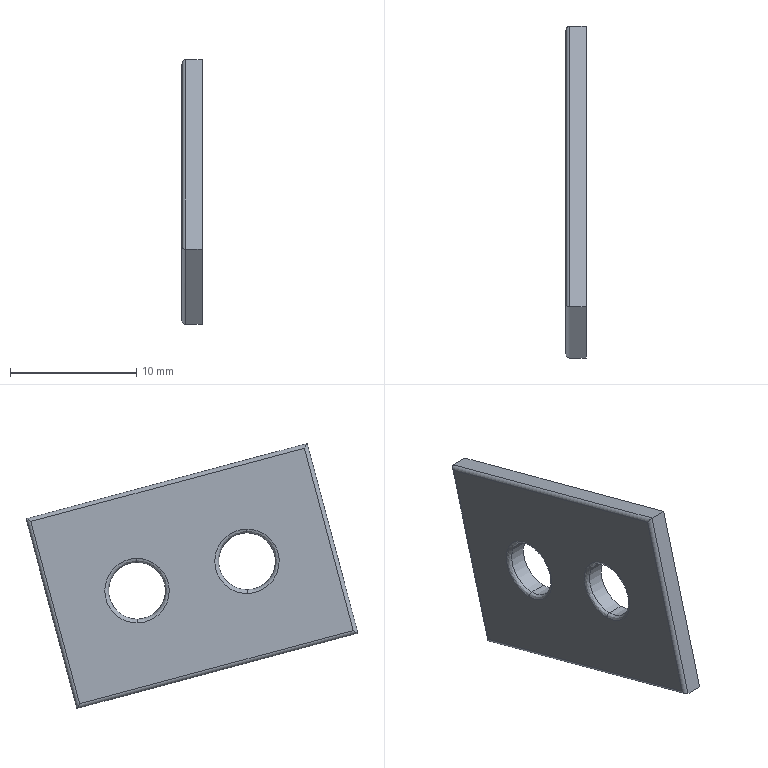Part | STEP file | Guide wheel mechanism revised.sldasm-Part-507 | 1 solid | 18 faces | box 1.6 x 26.233 x 20.944 mm | volume 518.202 mm3 | cylinder 8 | plane 6 | spline 4 | commonest cylinder face diameters 0.6 x4 4.5 x4
STEP:
#1=CARTESIAN_POINT('',(-1.3,8.693,-4.579));
#2=VERTEX_POINT('',#1);
#3=CARTESIAN_POINT('',(-1.3,8.699,-0.07938));
#4=VERTEX_POINT('',#3);
#5=CARTESIAN_POINT('',(-1.3,8.693,-2.329));
#6=DIRECTION('',(1.,0.,0.));
#7=DIRECTION('',(0.,0.,1.));
#8=AXIS2_PLACEMENT_3D('',#5,#6,#7);
#9=CIRCLE('',#8,2.25);
#10=EDGE_CURVE('',#2,#4,#9,.T.);
#11=ORIENTED_EDGE('',*,*,#10,.T.);
#12=CARTESIAN_POINT('',(-1.6,8.7,0.2206));
#13=VERTEX_POINT('',#12);
#14=CARTESIAN_POINT('',(-1.3,8.7,0.2206));
#15=DIRECTION('',(0.,1.,-0.002719));
#16=DIRECTION('',(0.,0.002719,1.));
#17=AXIS2_PLACEMENT_3D('',#14,#15,#16);
#18=CIRCLE('',#17,0.3);
#19=EDGE_CURVE('',#4,#13,#18,.T.);
#20=ORIENTED_EDGE('',*,*,#19,.T.);
#21=CARTESIAN_POINT('',(-1.6,8.693,-4.879));
#22=VERTEX_POINT('',#21);
#23=CARTESIAN_POINT('',(-1.6,8.7,0.2206));
#24=CARTESIAN_POINT('',(-1.6,13.786,0.2068));
#25=CARTESIAN_POINT('',(-1.6,13.779,-4.879));
#26=CARTESIAN_POINT('',(-1.6,8.693,-4.879));
#27=(BOUNDED_CURVE()B_SPLINE_CURVE(3,(#23,#24,#25,#26),.UNSPECIFIED.,.F.,.F.)B_SPLINE_CURVE_WITH_KNOTS((4,4),(0.0008654,1.),.UNSPECIFIED.)CURVE()GEOMETRIC_REPRESENTATION_ITEM()RATIONAL_B_SPLINE_CURVE((1.,0.3342,0.3342,1.))REPRESENTATION_ITEM(''));
#28=EDGE_CURVE('',#13,#22,#27,.T.);
#29=ORIENTED_EDGE('',*,*,#28,.T.);
#30=CARTESIAN_POINT('',(-1.6,8.686,-4.879));
#31=VERTEX_POINT('',#30);
#32=CARTESIAN_POINT('',(-1.6,8.693,-4.879));
#33=CARTESIAN_POINT('',(-1.6,8.691,-4.879));
#34=CARTESIAN_POINT('',(-1.6,8.689,-4.879));
#35=CARTESIAN_POINT('',(-1.6,8.686,-4.879));
#36=B_SPLINE_CURVE_WITH_KNOTS('',3,(#32,#33,#34,#35),.UNSPECIFIED.,.F.,.F.,(4,4),(0.,0.0008545),.UNSPECIFIED.);
#37=EDGE_CURVE('',#22,#31,#36,.T.);
#38=ORIENTED_EDGE('',*,*,#37,.T.);
#39=CARTESIAN_POINT('',(-1.3,8.687,-4.579));
#40=VERTEX_POINT('',#39);
#41=CARTESIAN_POINT('',(-1.3,8.686,-4.879));
#42=DIRECTION('',(0.,-1.,0.002719));
#43=DIRECTION('',(0.,-0.002719,-1.));
#44=AXIS2_PLACEMENT_3D('',#41,#42,#43);
#45=CIRCLE('',#44,0.3);
#46=EDGE_CURVE('',#40,#31,#45,.T.);
#47=ORIENTED_EDGE('',*,*,#46,.F.);
#48=CARTESIAN_POINT('',(-1.3,8.693,-2.329));
#49=DIRECTION('',(1.,0.,0.));
#50=DIRECTION('',(0.,0.,1.));
#51=AXIS2_PLACEMENT_3D('',#48,#49,#50);
#52=CIRCLE('',#51,2.25);
#53=EDGE_CURVE('',#40,#2,#52,.T.);
#54=ORIENTED_EDGE('',*,*,#53,.T.);
#55=EDGE_LOOP('',(#11,#20,#29,#38,#47,#54));
#56=FACE_OUTER_BOUND('',#55,.T.);
#57=CARTESIAN_POINT('',(-1.3,8.699,-0.07938));
#58=CARTESIAN_POINT('',(-1.3,10.017,-0.08296));
#59=CARTESIAN_POINT('',(-1.3,10.947,-1.017));
#60=CARTESIAN_POINT('',(-1.3,10.943,-2.335));
#61=CARTESIAN_POINT('',(-1.3,10.94,-3.654));
#62=CARTESIAN_POINT('',(-1.3,10.005,-4.583));
#63=CARTESIAN_POINT('',(-1.3,8.687,-4.579));
#64=CARTESIAN_POINT('',(-1.477,8.699,-0.07938));
#65=CARTESIAN_POINT('',(-1.477,10.017,-0.08296));
#66=CARTESIAN_POINT('',(-1.477,10.947,-1.017));
#67=CARTESIAN_POINT('',(-1.477,10.943,-2.335));
#68=CARTESIAN_POINT('',(-1.477,10.94,-3.654));
#69=CARTESIAN_POINT('',(-1.477,10.005,-4.583));
#70=CARTESIAN_POINT('',(-1.477,8.687,-4.579));
#71=CARTESIAN_POINT('',(-1.602,8.7,0.0464));
#72=CARTESIAN_POINT('',(-1.602,10.091,0.04262));
#73=CARTESIAN_POINT('',(-1.602,11.073,-0.9441));
#74=CARTESIAN_POINT('',(-1.602,11.069,-2.336));
#75=CARTESIAN_POINT('',(-1.602,11.065,-3.728));
#76=CARTESIAN_POINT('',(-1.602,10.079,-4.709));
#77=CARTESIAN_POINT('',(-1.602,8.687,-4.705));
#78=CARTESIAN_POINT('',(-1.6,8.7,0.2234));
#79=CARTESIAN_POINT('',(-1.6,10.196,0.2194));
#80=CARTESIAN_POINT('',(-1.6,11.25,-0.8409));
#81=CARTESIAN_POINT('',(-1.6,11.246,-2.336));
#82=CARTESIAN_POINT('',(-1.6,11.242,-3.832));
#83=CARTESIAN_POINT('',(-1.6,10.182,-4.886));
#84=CARTESIAN_POINT('',(-1.6,8.686,-4.882));
#85=(BOUNDED_SURFACE()B_SPLINE_SURFACE(3,3,((#57,#58,#59,#60,#61,#62,#63),(#64,#65,#66,#67,#68,#69,#70),(#71,#72,#73,#74,#75,#76,#77),(#78,#79,#80,#81,#82,#83,#84)),.UNSPECIFIED.,.F.,.F.,.F.)B_SPLINE_SURFACE_WITH_KNOTS((4,4),(4,3,4),(0.,1.),(0.,0.5,1.),.UNSPECIFIED.)GEOMETRIC_REPRESENTATION_ITEM()RATIONAL_B_SPLINE_SURFACE(((1.,0.8047,0.8047,1.,0.8047,0.8047,1.),(0.8025,0.6458,0.6458,0.8025,0.6458,0.6458,0.8025),(0.8025,0.6458,0.6458,0.8025,0.6458,0.6458,0.8025),(1.,0.8047,0.8047,1.,0.8047,0.8047,1.)))REPRESENTATION_ITEM('')SURFACE());
#86=ADVANCED_FACE('',(#56),#85,.T.);
#87=CARTESIAN_POINT('',(-1.3,0.,-2.25));
#88=VERTEX_POINT('',#87);
#89=CARTESIAN_POINT('',(-1.3,0.006117,2.25));
#90=VERTEX_POINT('',#89);
#91=CARTESIAN_POINT('',(-1.3,0.,0.));
#92=DIRECTION('',(1.,0.,0.));
#93=DIRECTION('',(0.,0.,1.));
#94=AXIS2_PLACEMENT_3D('',#91,#92,#93);
#95=CIRCLE('',#94,2.25);
#96=EDGE_CURVE('',#88,#90,#95,.T.);
#97=ORIENTED_EDGE('',*,*,#96,.T.);
#98=CARTESIAN_POINT('',(-1.6,0.006933,2.55));
#99=VERTEX_POINT('',#98);
#100=CARTESIAN_POINT('',(-1.3,0.006933,2.55));
#101=DIRECTION('',(0.,1.,-0.002719));
#102=DIRECTION('',(0.,0.002719,1.));
#103=AXIS2_PLACEMENT_3D('',#100,#101,#102);
#104=CIRCLE('',#103,0.3);
#105=EDGE_CURVE('',#90,#99,#104,.T.);
#106=ORIENTED_EDGE('',*,*,#105,.T.);
#107=CARTESIAN_POINT('',(-1.6,0.,-2.55));
#108=VERTEX_POINT('',#107);
#109=CARTESIAN_POINT('',(-1.6,0.006933,2.55));
#110=CARTESIAN_POINT('',(-1.6,5.093,2.536));
#111=CARTESIAN_POINT('',(-1.6,5.086,-2.55));
#112=CARTESIAN_POINT('',(-1.6,0.,-2.55));
#113=(BOUNDED_CURVE()B_SPLINE_CURVE(3,(#109,#110,#111,#112),.UNSPECIFIED.,.F.,.F.)B_SPLINE_CURVE_WITH_KNOTS((4,4),(0.0008654,1.),.UNSPECIFIED.)CURVE()GEOMETRIC_REPRESENTATION_ITEM()RATIONAL_B_SPLINE_CURVE((1.,0.3342,0.3342,1.))REPRESENTATION_ITEM(''));
#114=EDGE_CURVE('',#99,#108,#113,.T.);
#115=ORIENTED_EDGE('',*,*,#114,.T.);
#116=CARTESIAN_POINT('',(-1.6,-0.006933,-2.55));
#117=VERTEX_POINT('',#116);
#118=CARTESIAN_POINT('',(-1.6,0.,-2.55));
#119=CARTESIAN_POINT('',(-1.6,-0.002296,-2.55));
#120=CARTESIAN_POINT('',(-1.6,-0.004651,-2.55));
#121=CARTESIAN_POINT('',(-1.6,-0.006933,-2.55));
#122=B_SPLINE_CURVE_WITH_KNOTS('',3,(#118,#119,#120,#121),.UNSPECIFIED.,.F.,.F.,(4,4),(0.,0.0008545),.UNSPECIFIED.);
#123=EDGE_CURVE('',#108,#117,#122,.T.);
#124=ORIENTED_EDGE('',*,*,#123,.T.);
#125=CARTESIAN_POINT('',(-1.3,-0.006117,-2.25));
#126=VERTEX_POINT('',#125);
#127=CARTESIAN_POINT('',(-1.3,-0.006933,-2.55));
#128=DIRECTION('',(0.,-1.,0.002719));
#129=DIRECTION('',(0.,-0.002719,-1.));
#130=AXIS2_PLACEMENT_3D('',#127,#128,#129);
#131=CIRCLE('',#130,0.3);
#132=EDGE_CURVE('',#126,#117,#131,.T.);
#133=ORIENTED_EDGE('',*,*,#132,.F.);
#134=CARTESIAN_POINT('',(-1.3,0.,0.));
#135=DIRECTION('',(1.,0.,0.));
#136=DIRECTION('',(0.,0.,1.));
#137=AXIS2_PLACEMENT_3D('',#134,#135,#136);
#138=CIRCLE('',#137,2.25);
#139=EDGE_CURVE('',#126,#88,#138,.T.);
#140=ORIENTED_EDGE('',*,*,#139,.T.);
#141=EDGE_LOOP('',(#97,#106,#115,#124,#133,#140));
#142=FACE_OUTER_BOUND('',#141,.T.);
#143=CARTESIAN_POINT('',(-1.3,0.006117,2.25));
#144=CARTESIAN_POINT('',(-1.3,1.324,2.246));
#145=CARTESIAN_POINT('',(-1.3,2.254,1.312));
#146=CARTESIAN_POINT('',(-1.3,2.25,-0.006117));
#147=CARTESIAN_POINT('',(-1.3,2.246,-1.324));
#148=CARTESIAN_POINT('',(-1.3,1.312,-2.254));
#149=CARTESIAN_POINT('',(-1.3,-0.006117,-2.25));
#150=CARTESIAN_POINT('',(-1.477,0.006117,2.25));
#151=CARTESIAN_POINT('',(-1.477,1.324,2.246));
#152=CARTESIAN_POINT('',(-1.477,2.254,1.312));
#153=CARTESIAN_POINT('',(-1.477,2.25,-0.006117));
#154=CARTESIAN_POINT('',(-1.477,2.246,-1.324));
#155=CARTESIAN_POINT('',(-1.477,1.312,-2.254));
#156=CARTESIAN_POINT('',(-1.477,-0.006117,-2.25));
#157=CARTESIAN_POINT('',(-1.602,0.006459,2.376));
#158=CARTESIAN_POINT('',(-1.602,1.398,2.372));
#159=CARTESIAN_POINT('',(-1.602,2.38,1.385));
#160=CARTESIAN_POINT('',(-1.602,2.376,-0.006459));
#161=CARTESIAN_POINT('',(-1.602,2.372,-1.398));
#162=CARTESIAN_POINT('',(-1.602,1.385,-2.38));
#163=CARTESIAN_POINT('',(-1.602,-0.006459,-2.376));
#164=CARTESIAN_POINT('',(-1.6,0.00694,2.553));
#165=CARTESIAN_POINT('',(-1.6,1.502,2.549));
#166=CARTESIAN_POINT('',(-1.6,2.557,1.488));
#167=CARTESIAN_POINT('',(-1.6,2.553,-0.00694));
#168=CARTESIAN_POINT('',(-1.6,2.549,-1.502));
#169=CARTESIAN_POINT('',(-1.6,1.488,-2.557));
#170=CARTESIAN_POINT('',(-1.6,-0.00694,-2.553));
#171=(BOUNDED_SURFACE()B_SPLINE_SURFACE(3,3,((#143,#144,#145,#146,#147,#148,#149),(#150,#151,#152,#153,#154,#155,#156),(#157,#158,#159,#160,#161,#162,#163),(#164,#165,#166,#167,#168,#169,#170)),.UNSPECIFIED.,.F.,.F.,.F.)B_SPLINE_SURFACE_WITH_KNOTS((4,4),(4,3,4),(0.,1.),(0.,0.5,1.),.UNSPECIFIED.)GEOMETRIC_REPRESENTATION_ITEM()RATIONAL_B_SPLINE_SURFACE(((1.,0.8047,0.8047,1.,0.8047,0.8047,1.),(0.8025,0.6458,0.6458,0.8025,0.6458,0.6458,0.8025),(0.8025,0.6458,0.6458,0.8025,0.6458,0.6458,0.8025),(1.,0.8047,0.8047,1.,0.8047,0.8047,1.)))REPRESENTATION_ITEM('')SURFACE());
#172=ADVANCED_FACE('',(#142),#171,.T.);
#173=CARTESIAN_POINT('',(0.,8.693,-0.07937));
#174=VERTEX_POINT('',#173);
#175=CARTESIAN_POINT('',(0.,8.693,-4.579));
#176=VERTEX_POINT('',#175);
#177=CARTESIAN_POINT('',(0.,8.693,-2.329));
#178=DIRECTION('',(1.,0.,0.));
#179=DIRECTION('',(0.,0.,1.));
#180=AXIS2_PLACEMENT_3D('',#177,#178,#179);
#181=CIRCLE('',#180,2.25);
#182=EDGE_CURVE('',#174,#176,#181,.T.);
#183=ORIENTED_EDGE('',*,*,#182,.T.);
#184=CARTESIAN_POINT('',(0.,8.693,-4.579));
#185=DIRECTION('',(-1.,0.,0.));
#186=VECTOR('',#185,1000.);
#187=LINE('',#184,#186);
#188=EDGE_CURVE('',#176,#2,#187,.T.);
#189=ORIENTED_EDGE('',*,*,#188,.T.);
#190=ORIENTED_EDGE('',*,*,#53,.F.);
#191=CARTESIAN_POINT('',(-1.3,8.693,-0.07937));
#192=VERTEX_POINT('',#191);
#193=CARTESIAN_POINT('',(-1.3,8.693,-2.329));
#194=DIRECTION('',(1.,0.,0.));
#195=DIRECTION('',(0.,0.,1.));
#196=AXIS2_PLACEMENT_3D('',#193,#194,#195);
#197=CIRCLE('',#196,2.25);
#198=EDGE_CURVE('',#192,#40,#197,.T.);
#199=ORIENTED_EDGE('',*,*,#198,.F.);
#200=CARTESIAN_POINT('',(0.,8.693,-0.07937));
#201=DIRECTION('',(-1.,0.,0.));
#202=VECTOR('',#201,1000.);
#203=LINE('',#200,#202);
#204=EDGE_CURVE('',#174,#192,#203,.T.);
#205=ORIENTED_EDGE('',*,*,#204,.F.);
#206=EDGE_LOOP('',(#183,#189,#190,#199,#205));
#207=FACE_OUTER_BOUND('',#206,.T.);
#208=CARTESIAN_POINT('',(0.,8.693,-2.329));
#209=DIRECTION('',(-1.,0.,0.));
#210=DIRECTION('',(0.,0.,1.));
#211=AXIS2_PLACEMENT_3D('',#208,#209,#210);
#212=CYLINDRICAL_SURFACE('',#211,2.25);
#213=ADVANCED_FACE('',(#207),#212,.F.);
#214=CARTESIAN_POINT('',(0.,0.,2.25));
#215=VERTEX_POINT('',#214);
#216=CARTESIAN_POINT('',(0.,0.,-2.25));
#217=VERTEX_POINT('',#216);
#218=CARTESIAN_POINT('',(0.,0.,0.));
#219=DIRECTION('',(1.,0.,0.));
#220=DIRECTION('',(0.,0.,1.));
#221=AXIS2_PLACEMENT_3D('',#218,#219,#220);
#222=CIRCLE('',#221,2.25);
#223=EDGE_CURVE('',#215,#217,#222,.T.);
#224=ORIENTED_EDGE('',*,*,#223,.T.);
#225=CARTESIAN_POINT('',(0.,0.,-2.25));
#226=DIRECTION('',(-1.,0.,0.));
#227=VECTOR('',#226,1000.);
#228=LINE('',#225,#227);
#229=EDGE_CURVE('',#217,#88,#228,.T.);
#230=ORIENTED_EDGE('',*,*,#229,.T.);
#231=ORIENTED_EDGE('',*,*,#139,.F.);
#232=CARTESIAN_POINT('',(-1.3,0.,2.25));
#233=VERTEX_POINT('',#232);
#234=CARTESIAN_POINT('',(-1.3,0.,0.));
#235=DIRECTION('',(1.,0.,0.));
#236=DIRECTION('',(0.,0.,1.));
#237=AXIS2_PLACEMENT_3D('',#234,#235,#236);
#238=CIRCLE('',#237,2.25);
#239=EDGE_CURVE('',#233,#126,#238,.T.);
#240=ORIENTED_EDGE('',*,*,#239,.F.);
#241=CARTESIAN_POINT('',(0.,0.,2.25));
#242=DIRECTION('',(-1.,0.,0.));
#243=VECTOR('',#242,1000.);
#244=LINE('',#241,#243);
#245=EDGE_CURVE('',#215,#233,#244,.T.);
#246=ORIENTED_EDGE('',*,*,#245,.F.);
#247=EDGE_LOOP('',(#224,#230,#231,#240,#246));
#248=FACE_OUTER_BOUND('',#247,.T.);
#249=CARTESIAN_POINT('',(0.,0.,0.));
#250=DIRECTION('',(-1.,0.,0.));
#251=DIRECTION('',(0.,0.,1.));
#252=AXIS2_PLACEMENT_3D('',#249,#250,#251);
#253=CYLINDRICAL_SURFACE('',#252,2.25);
#254=ADVANCED_FACE('',(#248),#253,.F.);
#255=ORIENTED_EDGE('',*,*,#182,.F.);
#256=CARTESIAN_POINT('',(0.,8.693,-2.329));
#257=DIRECTION('',(1.,0.,0.));
#258=DIRECTION('',(0.,0.,1.));
#259=AXIS2_PLACEMENT_3D('',#256,#257,#258);
#260=CIRCLE('',#259,2.25);
#261=EDGE_CURVE('',#176,#174,#260,.T.);
#262=ORIENTED_EDGE('',*,*,#261,.F.);
#263=EDGE_LOOP('',(#255,#262));
#264=FACE_BOUND('',#263,.T.);
#265=ORIENTED_EDGE('',*,*,#223,.F.);
#266=CARTESIAN_POINT('',(0.,0.,0.));
#267=DIRECTION('',(1.,0.,0.));
#268=DIRECTION('',(0.,0.,1.));
#269=AXIS2_PLACEMENT_3D('',#266,#267,#268);
#270=CIRCLE('',#269,2.25);
#271=EDGE_CURVE('',#217,#215,#270,.T.);
#272=ORIENTED_EDGE('',*,*,#271,.F.);
#273=EDGE_LOOP('',(#265,#272));
#274=FACE_BOUND('',#273,.T.);
#275=CARTESIAN_POINT('',(0.,-4.753,9.307));
#276=VERTEX_POINT('',#275);
#277=CARTESIAN_POINT('',(0.,17.463,3.354));
#278=VERTEX_POINT('',#277);
#279=CARTESIAN_POINT('',(0.,-4.753,9.307));
#280=DIRECTION('',(0.,0.9659,-0.2588));
#281=VECTOR('',#280,1000.);
#282=LINE('',#279,#281);
#283=EDGE_CURVE('',#276,#278,#282,.T.);
#284=ORIENTED_EDGE('',*,*,#283,.F.);
#285=CARTESIAN_POINT('',(0.,-8.77,-5.684));
#286=VERTEX_POINT('',#285);
#287=CARTESIAN_POINT('',(0.,-8.77,-5.684));
#288=DIRECTION('',(0.,0.2588,0.9659));
#289=VECTOR('',#288,1000.);
#290=LINE('',#287,#289);
#291=EDGE_CURVE('',#286,#276,#290,.T.);
#292=ORIENTED_EDGE('',*,*,#291,.F.);
#293=CARTESIAN_POINT('',(0.,13.446,-11.637));
#294=VERTEX_POINT('',#293);
#295=CARTESIAN_POINT('',(0.,13.446,-11.637));
#296=DIRECTION('',(0.,-0.9659,0.2588));
#297=VECTOR('',#296,1000.);
#298=LINE('',#295,#297);
#299=EDGE_CURVE('',#294,#286,#298,.T.);
#300=ORIENTED_EDGE('',*,*,#299,.F.);
#301=CARTESIAN_POINT('',(0.,17.463,3.354));
#302=DIRECTION('',(0.,-0.2588,-0.9659));
#303=VECTOR('',#302,1000.);
#304=LINE('',#301,#303);
#305=EDGE_CURVE('',#278,#294,#304,.T.);
#306=ORIENTED_EDGE('',*,*,#305,.F.);
#307=EDGE_LOOP('',(#284,#292,#300,#306));
#308=FACE_OUTER_BOUND('',#307,.T.);
#309=CARTESIAN_POINT('',(0.,0.,0.));
#310=DIRECTION('',(-1.,0.,0.));
#311=DIRECTION('',(0.,0.,1.));
#312=AXIS2_PLACEMENT_3D('',#309,#310,#311);
#313=PLANE('',#312);
#314=ADVANCED_FACE('',(#264,#274,#308),#313,.F.);
#315=ORIENTED_EDGE('',*,*,#188,.F.);
#316=ORIENTED_EDGE('',*,*,#261,.T.);
#317=ORIENTED_EDGE('',*,*,#204,.T.);
#318=CARTESIAN_POINT('',(-1.3,8.693,-2.329));
#319=DIRECTION('',(1.,0.,0.));
#320=DIRECTION('',(0.,0.,1.));
#321=AXIS2_PLACEMENT_3D('',#318,#319,#320);
#322=CIRCLE('',#321,2.25);
#323=EDGE_CURVE('',#4,#192,#322,.T.);
#324=ORIENTED_EDGE('',*,*,#323,.F.);
#325=ORIENTED_EDGE('',*,*,#10,.F.);
#326=EDGE_LOOP('',(#315,#316,#317,#324,#325));
#327=FACE_OUTER_BOUND('',#326,.T.);
#328=CARTESIAN_POINT('',(0.,8.693,-2.329));
#329=DIRECTION('',(-1.,0.,0.));
#330=DIRECTION('',(0.,0.,1.));
#331=AXIS2_PLACEMENT_3D('',#328,#329,#330);
#332=CYLINDRICAL_SURFACE('',#331,2.25);
#333=ADVANCED_FACE('',(#327),#332,.F.);
#334=ORIENTED_EDGE('',*,*,#229,.F.);
#335=ORIENTED_EDGE('',*,*,#271,.T.);
#336=ORIENTED_EDGE('',*,*,#245,.T.);
#337=CARTESIAN_POINT('',(-1.3,0.,0.));
#338=DIRECTION('',(1.,0.,0.));
#339=DIRECTION('',(0.,0.,1.));
#340=AXIS2_PLACEMENT_3D('',#337,#338,#339);
#341=CIRCLE('',#340,2.25);
#342=EDGE_CURVE('',#90,#233,#341,.T.);
#343=ORIENTED_EDGE('',*,*,#342,.F.);
#344=ORIENTED_EDGE('',*,*,#96,.F.);
#345=EDGE_LOOP('',(#334,#335,#336,#343,#344));
#346=FACE_OUTER_BOUND('',#345,.T.);
#347=CARTESIAN_POINT('',(0.,0.,0.));
#348=DIRECTION('',(-1.,0.,0.));
#349=DIRECTION('',(0.,0.,1.));
#350=AXIS2_PLACEMENT_3D('',#347,#348,#349);
#351=CYLINDRICAL_SURFACE('',#350,2.25);
#352=ADVANCED_FACE('',(#346),#351,.F.);
#353=CARTESIAN_POINT('',(-1.3,13.446,-11.637));
#354=VERTEX_POINT('',#353);
#355=CARTESIAN_POINT('',(0.,13.446,-11.637));
#356=DIRECTION('',(-1.,0.,0.));
#357=VECTOR('',#356,1000.);
#358=LINE('',#355,#357);
#359=EDGE_CURVE('',#294,#354,#358,.T.);
#360=ORIENTED_EDGE('',*,*,#359,.T.);
#361=CARTESIAN_POINT('',(-1.3,17.463,3.354));
#362=VERTEX_POINT('',#361);
#363=CARTESIAN_POINT('',(-1.3,17.463,3.354));
#364=DIRECTION('',(0.,0.2588,0.9659));
#365=VECTOR('',#364,1000.);
#366=LINE('',#363,#365);
#367=EDGE_CURVE('',#354,#362,#366,.T.);
#368=ORIENTED_EDGE('',*,*,#367,.T.);
#369=CARTESIAN_POINT('',(0.,17.463,3.354));
#370=DIRECTION('',(1.,0.,0.));
#371=VECTOR('',#370,1000.);
#372=LINE('',#369,#371);
#373=EDGE_CURVE('',#362,#278,#372,.T.);
#374=ORIENTED_EDGE('',*,*,#373,.T.);
#375=ORIENTED_EDGE('',*,*,#305,.T.);
#376=EDGE_LOOP('',(#360,#368,#374,#375));
#377=FACE_OUTER_BOUND('',#376,.T.);
#378=CARTESIAN_POINT('',(0.,17.463,3.354));
#379=DIRECTION('',(0.,0.9659,-0.2588));
#380=DIRECTION('',(0.,0.2588,0.9659));
#381=AXIS2_PLACEMENT_3D('',#378,#379,#380);
#382=PLANE('',#381);
#383=ADVANCED_FACE('',(#377),#382,.T.);
#384=ORIENTED_EDGE('',*,*,#373,.F.);
#385=CARTESIAN_POINT('',(-1.3,-4.753,9.307));
#386=VERTEX_POINT('',#385);
#387=CARTESIAN_POINT('',(-1.3,-4.753,9.307));
#388=DIRECTION('',(0.,-0.9659,0.2588));
#389=VECTOR('',#388,1000.);
#390=LINE('',#387,#389);
#391=EDGE_CURVE('',#362,#386,#390,.T.);
#392=ORIENTED_EDGE('',*,*,#391,.T.);
#393=CARTESIAN_POINT('',(0.,-4.753,9.307));
#394=DIRECTION('',(1.,0.,0.));
#395=VECTOR('',#394,1000.);
#396=LINE('',#393,#395);
#397=EDGE_CURVE('',#386,#276,#396,.T.);
#398=ORIENTED_EDGE('',*,*,#397,.T.);
#399=ORIENTED_EDGE('',*,*,#283,.T.);
#400=EDGE_LOOP('',(#384,#392,#398,#399));
#401=FACE_OUTER_BOUND('',#400,.T.);
#402=CARTESIAN_POINT('',(0.,-4.753,9.307));
#403=DIRECTION('',(0.,0.2588,0.9659));
#404=DIRECTION('',(0.,-0.9659,0.2588));
#405=AXIS2_PLACEMENT_3D('',#402,#403,#404);
#406=PLANE('',#405);
#407=ADVANCED_FACE('',(#401),#406,.T.);
#408=ORIENTED_EDGE('',*,*,#397,.F.);
#409=CARTESIAN_POINT('',(-1.3,-8.77,-5.684));
#410=VERTEX_POINT('',#409);
#411=CARTESIAN_POINT('',(-1.3,-8.77,-5.684));
#412=DIRECTION('',(0.,-0.2588,-0.9659));
#413=VECTOR('',#412,1000.);
#414=LINE('',#411,#413);
#415=EDGE_CURVE('',#386,#410,#414,.T.);
#416=ORIENTED_EDGE('',*,*,#415,.T.);
#417=CARTESIAN_POINT('',(0.,-8.77,-5.684));
#418=DIRECTION('',(1.,0.,0.));
#419=VECTOR('',#418,1000.);
#420=LINE('',#417,#419);
#421=EDGE_CURVE('',#410,#286,#420,.T.);
#422=ORIENTED_EDGE('',*,*,#421,.T.);
#423=ORIENTED_EDGE('',*,*,#291,.T.);
#424=EDGE_LOOP('',(#408,#416,#422,#423));
#425=FACE_OUTER_BOUND('',#424,.T.);
#426=CARTESIAN_POINT('',(0.,-8.77,-5.684));
#427=DIRECTION('',(0.,-0.9659,0.2588));
#428=DIRECTION('',(0.,-0.2588,-0.9659));
#429=AXIS2_PLACEMENT_3D('',#426,#427,#428);
#430=PLANE('',#429);
#431=ADVANCED_FACE('',(#425),#430,.T.);
#432=ORIENTED_EDGE('',*,*,#421,.F.);
#433=CARTESIAN_POINT('',(-1.3,13.446,-11.637));
#434=DIRECTION('',(0.,0.9659,-0.2588));
#435=VECTOR('',#434,1000.);
#436=LINE('',#433,#435);
#437=EDGE_CURVE('',#410,#354,#436,.T.);
#438=ORIENTED_EDGE('',*,*,#437,.T.);
#439=ORIENTED_EDGE('',*,*,#359,.F.);
#440=ORIENTED_EDGE('',*,*,#299,.T.);
#441=EDGE_LOOP('',(#432,#438,#439,#440));
#442=FACE_OUTER_BOUND('',#441,.T.);
#443=CARTESIAN_POINT('',(0.,13.446,-11.637));
#444=DIRECTION('',(0.,-0.2588,-0.9659));
#445=DIRECTION('',(0.,0.9659,-0.2588));
#446=AXIS2_PLACEMENT_3D('',#443,#444,#445);
#447=PLANE('',#446);
#448=ADVANCED_FACE('',(#442),#447,.T.);
#449=ORIENTED_EDGE('',*,*,#19,.F.);
#450=ORIENTED_EDGE('',*,*,#323,.T.);
#451=ORIENTED_EDGE('',*,*,#198,.T.);
#452=ORIENTED_EDGE('',*,*,#46,.T.);
#453=CARTESIAN_POINT('',(-1.6,8.693,0.2206));
#454=VERTEX_POINT('',#453);
#455=CARTESIAN_POINT('',(-1.6,8.686,-4.879));
#456=CARTESIAN_POINT('',(-1.6,8.353,-4.878));
#457=CARTESIAN_POINT('',(-1.6,8.02,-4.811));
#458=CARTESIAN_POINT('',(-1.6,7.404,-4.555));
#459=CARTESIAN_POINT('',(-1.6,7.122,-4.365));
#460=CARTESIAN_POINT('',(-1.6,6.651,-3.893));
#461=CARTESIAN_POINT('',(-1.6,6.463,-3.61));
#462=CARTESIAN_POINT('',(-1.6,6.209,-2.993));
#463=CARTESIAN_POINT('',(-1.6,6.143,-2.659));
#464=CARTESIAN_POINT('',(-1.6,6.144,-1.992));
#465=CARTESIAN_POINT('',(-1.6,6.21,-1.659));
#466=CARTESIAN_POINT('',(-1.6,6.466,-1.043));
#467=CARTESIAN_POINT('',(-1.6,6.655,-0.7606));
#468=CARTESIAN_POINT('',(-1.6,7.127,-0.2893));
#469=CARTESIAN_POINT('',(-1.6,7.41,-0.1006));
#470=CARTESIAN_POINT('',(-1.6,8.026,0.1544));
#471=CARTESIAN_POINT('',(-1.6,8.36,0.2206));
#472=CARTESIAN_POINT('',(-1.6,8.693,0.2206));
#473=B_SPLINE_CURVE_WITH_KNOTS('',3,(#455,#456,#457,#458,#459,#460,#461,#462,#463,#464,#465,#466,#467,#468,#469,#470,#471,#472),.UNSPECIFIED.,.F.,.F.,(4,2,2,2,2,2,2,2,4),(0.0008545,0.1257,0.2506,0.3755,0.5004,0.6253,0.7502,0.8751,1.),.UNSPECIFIED.);
#474=EDGE_CURVE('',#31,#454,#473,.T.);
#475=ORIENTED_EDGE('',*,*,#474,.T.);
#476=CARTESIAN_POINT('',(-1.6,8.693,0.2206));
#477=CARTESIAN_POINT('',(-1.6,8.696,0.2206));
#478=CARTESIAN_POINT('',(-1.6,8.698,0.2206));
#479=CARTESIAN_POINT('',(-1.6,8.7,0.2206));
#480=(BOUNDED_CURVE()B_SPLINE_CURVE(3,(#476,#477,#478,#479),.UNSPECIFIED.,.F.,.F.)B_SPLINE_CURVE_WITH_KNOTS((4,4),(0.,0.0008654),.UNSPECIFIED.)CURVE()GEOMETRIC_REPRESENTATION_ITEM()RATIONAL_B_SPLINE_CURVE((1.,1.,1.,1.))REPRESENTATION_ITEM(''));
#481=EDGE_CURVE('',#454,#13,#480,.T.);
#482=ORIENTED_EDGE('',*,*,#481,.T.);
#483=EDGE_LOOP('',(#449,#450,#451,#452,#475,#482));
#484=FACE_OUTER_BOUND('',#483,.T.);
#485=CARTESIAN_POINT('',(-1.3,8.687,-4.579));
#486=CARTESIAN_POINT('',(-1.3,4.187,-4.567));
#487=CARTESIAN_POINT('',(-1.3,4.199,-0.06715));
#488=CARTESIAN_POINT('',(-1.3,8.699,-0.07938));
#489=CARTESIAN_POINT('',(-1.477,8.687,-4.579));
#490=CARTESIAN_POINT('',(-1.477,4.187,-4.567));
#491=CARTESIAN_POINT('',(-1.477,4.199,-0.06715));
#492=CARTESIAN_POINT('',(-1.477,8.699,-0.07938));
#493=CARTESIAN_POINT('',(-1.602,8.687,-4.705));
#494=CARTESIAN_POINT('',(-1.602,3.935,-4.692));
#495=CARTESIAN_POINT('',(-1.602,3.948,0.05945));
#496=CARTESIAN_POINT('',(-1.602,8.7,0.04653));
#497=CARTESIAN_POINT('',(-1.6,8.686,-4.882));
#498=CARTESIAN_POINT('',(-1.6,3.58,-4.869));
#499=CARTESIAN_POINT('',(-1.6,3.594,0.2376));
#500=CARTESIAN_POINT('',(-1.6,8.7,0.2237));
#501=(BOUNDED_SURFACE()B_SPLINE_SURFACE(3,3,((#485,#486,#487,#488),(#489,#490,#491,#492),(#493,#494,#495,#496),(#497,#498,#499,#500)),.UNSPECIFIED.,.F.,.F.,.T.)B_SPLINE_SURFACE_WITH_KNOTS((4,4),(4,4),(0.,1.),(0.,1.),.UNSPECIFIED.)GEOMETRIC_REPRESENTATION_ITEM()RATIONAL_B_SPLINE_SURFACE(((1.,0.3333,0.3333,1.),(0.8023,0.2674,0.2674,0.8023),(0.8023,0.2674,0.2674,0.8023),(1.,0.3333,0.3333,1.)))REPRESENTATION_ITEM('')SURFACE());
#502=ADVANCED_FACE('',(#484),#501,.T.);
#503=ORIENTED_EDGE('',*,*,#105,.F.);
#504=ORIENTED_EDGE('',*,*,#342,.T.);
#505=ORIENTED_EDGE('',*,*,#239,.T.);
#506=ORIENTED_EDGE('',*,*,#132,.T.);
#507=CARTESIAN_POINT('',(-1.6,0.,2.55));
#508=VERTEX_POINT('',#507);
#509=CARTESIAN_POINT('',(-1.6,-0.006933,-2.55));
#510=CARTESIAN_POINT('',(-1.6,-0.3404,-2.549));
#511=CARTESIAN_POINT('',(-1.6,-0.6736,-2.482));
#512=CARTESIAN_POINT('',(-1.6,-1.289,-2.225));
#513=CARTESIAN_POINT('',(-1.6,-1.571,-2.036));
#514=CARTESIAN_POINT('',(-1.6,-2.042,-1.563));
#515=CARTESIAN_POINT('',(-1.6,-2.231,-1.28));
#516=CARTESIAN_POINT('',(-1.6,-2.485,-0.6635));
#517=CARTESIAN_POINT('',(-1.6,-2.551,-0.3301));
#518=CARTESIAN_POINT('',(-1.6,-2.55,0.337));
#519=CARTESIAN_POINT('',(-1.6,-2.483,0.6703));
#520=CARTESIAN_POINT('',(-1.6,-2.227,1.286));
#521=CARTESIAN_POINT('',(-1.6,-2.038,1.569));
#522=CARTESIAN_POINT('',(-1.6,-1.566,2.04));
#523=CARTESIAN_POINT('',(-1.6,-1.283,2.229));
#524=CARTESIAN_POINT('',(-1.6,-0.6669,2.484));
#525=CARTESIAN_POINT('',(-1.6,-0.3335,2.55));
#526=CARTESIAN_POINT('',(-1.6,0.,2.55));
#527=B_SPLINE_CURVE_WITH_KNOTS('',3,(#509,#510,#511,#512,#513,#514,#515,#516,#517,#518,#519,#520,#521,#522,#523,#524,#525,#526),.UNSPECIFIED.,.F.,.F.,(4,2,2,2,2,2,2,2,4),(0.0008545,0.1257,0.2506,0.3755,0.5004,0.6253,0.7502,0.8751,1.),.UNSPECIFIED.);
#528=EDGE_CURVE('',#117,#508,#527,.T.);
#529=ORIENTED_EDGE('',*,*,#528,.T.);
#530=CARTESIAN_POINT('',(-1.6,0.,2.55));
#531=CARTESIAN_POINT('',(-1.6,0.002311,2.55));
#532=CARTESIAN_POINT('',(-1.6,0.004622,2.55));
#533=CARTESIAN_POINT('',(-1.6,0.006933,2.55));
#534=(BOUNDED_CURVE()B_SPLINE_CURVE(3,(#530,#531,#532,#533),.UNSPECIFIED.,.F.,.F.)B_SPLINE_CURVE_WITH_KNOTS((4,4),(0.,0.0008654),.UNSPECIFIED.)CURVE()GEOMETRIC_REPRESENTATION_ITEM()RATIONAL_B_SPLINE_CURVE((1.,1.,1.,1.))REPRESENTATION_ITEM(''));
#535=EDGE_CURVE('',#508,#99,#534,.T.);
#536=ORIENTED_EDGE('',*,*,#535,.T.);
#537=EDGE_LOOP('',(#503,#504,#505,#506,#529,#536));
#538=FACE_OUTER_BOUND('',#537,.T.);
#539=CARTESIAN_POINT('',(-1.3,-0.006117,-2.25));
#540=CARTESIAN_POINT('',(-1.3,-4.506,-2.238));
#541=CARTESIAN_POINT('',(-1.3,-4.494,2.262));
#542=CARTESIAN_POINT('',(-1.3,0.006117,2.25));
#543=CARTESIAN_POINT('',(-1.477,-0.006117,-2.25));
#544=CARTESIAN_POINT('',(-1.477,-4.506,-2.238));
#545=CARTESIAN_POINT('',(-1.477,-4.494,2.262));
#546=CARTESIAN_POINT('',(-1.477,0.006117,2.25));
#547=CARTESIAN_POINT('',(-1.602,-0.006459,-2.376));
#548=CARTESIAN_POINT('',(-1.602,-4.758,-2.363));
#549=CARTESIAN_POINT('',(-1.602,-4.745,2.389));
#550=CARTESIAN_POINT('',(-1.602,0.006459,2.376));
#551=CARTESIAN_POINT('',(-1.6,-0.006941,-2.553));
#552=CARTESIAN_POINT('',(-1.6,-5.113,-2.539));
#553=CARTESIAN_POINT('',(-1.6,-5.099,2.567));
#554=CARTESIAN_POINT('',(-1.6,0.006941,2.553));
#555=(BOUNDED_SURFACE()B_SPLINE_SURFACE(3,3,((#539,#540,#541,#542),(#543,#544,#545,#546),(#547,#548,#549,#550),(#551,#552,#553,#554)),.UNSPECIFIED.,.F.,.F.,.F.)B_SPLINE_SURFACE_WITH_KNOTS((4,4),(4,4),(0.,1.),(0.,1.),.UNSPECIFIED.)GEOMETRIC_REPRESENTATION_ITEM()RATIONAL_B_SPLINE_SURFACE(((1.,0.3333,0.3333,1.),(0.8023,0.2674,0.2674,0.8023),(0.8023,0.2674,0.2674,0.8023),(1.,0.3333,0.3333,1.)))REPRESENTATION_ITEM('')SURFACE());
#556=ADVANCED_FACE('',(#538),#555,.T.);
#557=CARTESIAN_POINT('',(-1.6,13.234,-11.269));
#558=VERTEX_POINT('',#557);
#559=CARTESIAN_POINT('',(-1.3,13.446,-11.637));
#560=CARTESIAN_POINT('',(-1.476,13.446,-11.637));
#561=CARTESIAN_POINT('',(-1.6,13.359,-11.484));
#562=CARTESIAN_POINT('',(-1.6,13.234,-11.269));
#563=(BOUNDED_CURVE()B_SPLINE_CURVE(3,(#559,#560,#561,#562),.UNSPECIFIED.,.F.,.F.)B_SPLINE_CURVE_WITH_KNOTS((4,4),(0.,1.571),.UNSPECIFIED.)CURVE()GEOMETRIC_REPRESENTATION_ITEM()RATIONAL_B_SPLINE_CURVE((1.,0.8047,0.8047,1.))REPRESENTATION_ITEM(''));
#564=EDGE_CURVE('',#354,#558,#563,.T.);
#565=ORIENTED_EDGE('',*,*,#564,.T.);
#566=CARTESIAN_POINT('',(-1.6,17.096,3.142));
#567=VERTEX_POINT('',#566);
#568=CARTESIAN_POINT('',(-1.6,17.175,3.436));
#569=DIRECTION('',(0.,0.2588,0.9659));
#570=VECTOR('',#569,1000.);
#571=LINE('',#568,#570);
#572=EDGE_CURVE('',#558,#567,#571,.T.);
#573=ORIENTED_EDGE('',*,*,#572,.T.);
#574=CARTESIAN_POINT('',(-1.6,17.096,3.142));
#575=CARTESIAN_POINT('',(-1.6,17.311,3.267));
#576=CARTESIAN_POINT('',(-1.476,17.463,3.354));
#577=CARTESIAN_POINT('',(-1.3,17.463,3.354));
#578=(BOUNDED_CURVE()B_SPLINE_CURVE(3,(#574,#575,#576,#577),.UNSPECIFIED.,.F.,.T.)B_SPLINE_CURVE_WITH_KNOTS((4,4),(1.571,3.142),.UNSPECIFIED.)CURVE()GEOMETRIC_REPRESENTATION_ITEM()RATIONAL_B_SPLINE_CURVE((1.,0.8047,0.8047,1.))REPRESENTATION_ITEM(''));
#579=EDGE_CURVE('',#567,#362,#578,.T.);
#580=ORIENTED_EDGE('',*,*,#579,.T.);
#581=ORIENTED_EDGE('',*,*,#367,.F.);
#582=EDGE_LOOP('',(#565,#573,#580,#581));
#583=FACE_OUTER_BOUND('',#582,.T.);
#584=CARTESIAN_POINT('',(-1.3,17.175,3.436));
#585=DIRECTION('',(0.,-0.2588,-0.9659));
#586=DIRECTION('',(0.,0.9659,-0.2588));
#587=AXIS2_PLACEMENT_3D('',#584,#585,#586);
#588=CYLINDRICAL_SURFACE('',#587,0.3);
#589=ADVANCED_FACE('',(#583),#588,.T.);
#590=CARTESIAN_POINT('',(-1.6,-4.541,8.94));
#591=VERTEX_POINT('',#590);
#592=CARTESIAN_POINT('',(-1.6,-4.541,8.94));
#593=CARTESIAN_POINT('',(-1.6,-4.665,9.155));
#594=CARTESIAN_POINT('',(-1.476,-4.753,9.307));
#595=CARTESIAN_POINT('',(-1.3,-4.753,9.307));
#596=(BOUNDED_CURVE()B_SPLINE_CURVE(3,(#592,#593,#594,#595),.UNSPECIFIED.,.F.,.F.)B_SPLINE_CURVE_WITH_KNOTS((4,4),(1.571,3.142),.UNSPECIFIED.)CURVE()GEOMETRIC_REPRESENTATION_ITEM()RATIONAL_B_SPLINE_CURVE((1.,0.8047,0.8047,1.))REPRESENTATION_ITEM(''));
#597=EDGE_CURVE('',#591,#386,#596,.T.);
#598=ORIENTED_EDGE('',*,*,#597,.T.);
#599=ORIENTED_EDGE('',*,*,#391,.F.);
#600=ORIENTED_EDGE('',*,*,#579,.F.);
#601=CARTESIAN_POINT('',(-1.6,-4.835,9.019));
#602=DIRECTION('',(0.,-0.9659,0.2588));
#603=VECTOR('',#602,1000.);
#604=LINE('',#601,#603);
#605=EDGE_CURVE('',#567,#591,#604,.T.);
#606=ORIENTED_EDGE('',*,*,#605,.T.);
#607=EDGE_LOOP('',(#598,#599,#600,#606));
#608=FACE_OUTER_BOUND('',#607,.T.);
#609=CARTESIAN_POINT('',(-1.3,-4.835,9.019));
#610=DIRECTION('',(0.,0.9659,-0.2588));
#611=DIRECTION('',(0.,0.2588,0.9659));
#612=AXIS2_PLACEMENT_3D('',#609,#610,#611);
#613=CYLINDRICAL_SURFACE('',#612,0.3);
#614=ADVANCED_FACE('',(#608),#613,.T.);
#615=CARTESIAN_POINT('',(-1.6,-8.402,-5.472));
#616=VERTEX_POINT('',#615);
#617=CARTESIAN_POINT('',(-1.6,-8.402,-5.472));
#618=CARTESIAN_POINT('',(-1.6,-8.618,-5.596));
#619=CARTESIAN_POINT('',(-1.476,-8.77,-5.684));
#620=CARTESIAN_POINT('',(-1.3,-8.77,-5.684));
#621=(BOUNDED_CURVE()B_SPLINE_CURVE(3,(#617,#618,#619,#620),.UNSPECIFIED.,.F.,.F.)B_SPLINE_CURVE_WITH_KNOTS((4,4),(1.571,3.142),.UNSPECIFIED.)CURVE()GEOMETRIC_REPRESENTATION_ITEM()RATIONAL_B_SPLINE_CURVE((1.,0.8047,0.8047,1.))REPRESENTATION_ITEM(''));
#622=EDGE_CURVE('',#616,#410,#621,.T.);
#623=ORIENTED_EDGE('',*,*,#622,.T.);
#624=ORIENTED_EDGE('',*,*,#415,.F.);
#625=ORIENTED_EDGE('',*,*,#597,.F.);
#626=CARTESIAN_POINT('',(-1.6,-8.481,-5.766));
#627=DIRECTION('',(0.,-0.2588,-0.9659));
#628=VECTOR('',#627,1000.);
#629=LINE('',#626,#628);
#630=EDGE_CURVE('',#591,#616,#629,.T.);
#631=ORIENTED_EDGE('',*,*,#630,.T.);
#632=EDGE_LOOP('',(#623,#624,#625,#631));
#633=FACE_OUTER_BOUND('',#632,.T.);
#634=CARTESIAN_POINT('',(-1.3,-8.481,-5.766));
#635=DIRECTION('',(0.,0.2588,0.9659));
#636=DIRECTION('',(0.,-0.9659,0.2588));
#637=AXIS2_PLACEMENT_3D('',#634,#635,#636);
#638=CYLINDRICAL_SURFACE('',#637,0.3);
#639=ADVANCED_FACE('',(#633),#638,.T.);
#640=ORIENTED_EDGE('',*,*,#564,.F.);
#641=ORIENTED_EDGE('',*,*,#437,.F.);
#642=ORIENTED_EDGE('',*,*,#622,.F.);
#643=CARTESIAN_POINT('',(-1.6,13.528,-11.348));
#644=DIRECTION('',(0.,0.9659,-0.2588));
#645=VECTOR('',#644,1000.);
#646=LINE('',#643,#645);
#647=EDGE_CURVE('',#616,#558,#646,.T.);
#648=ORIENTED_EDGE('',*,*,#647,.T.);
#649=EDGE_LOOP('',(#640,#641,#642,#648));
#650=FACE_OUTER_BOUND('',#649,.T.);
#651=CARTESIAN_POINT('',(-1.3,13.528,-11.348));
#652=DIRECTION('',(0.,-0.9659,0.2588));
#653=DIRECTION('',(0.,-0.2588,-0.9659));
#654=AXIS2_PLACEMENT_3D('',#651,#652,#653);
#655=CYLINDRICAL_SURFACE('',#654,0.3);
#656=ADVANCED_FACE('',(#650),#655,.T.);
#657=ORIENTED_EDGE('',*,*,#37,.F.);
#658=ORIENTED_EDGE('',*,*,#28,.F.);
#659=ORIENTED_EDGE('',*,*,#481,.F.);
#660=ORIENTED_EDGE('',*,*,#474,.F.);
#661=EDGE_LOOP('',(#657,#658,#659,#660));
#662=FACE_BOUND('',#661,.T.);
#663=ORIENTED_EDGE('',*,*,#535,.F.);
#664=ORIENTED_EDGE('',*,*,#528,.F.);
#665=ORIENTED_EDGE('',*,*,#123,.F.);
#666=ORIENTED_EDGE('',*,*,#114,.F.);
#667=EDGE_LOOP('',(#663,#664,#665,#666));
#668=FACE_BOUND('',#667,.T.);
#669=ORIENTED_EDGE('',*,*,#630,.F.);
#670=ORIENTED_EDGE('',*,*,#605,.F.);
#671=ORIENTED_EDGE('',*,*,#572,.F.);
#672=ORIENTED_EDGE('',*,*,#647,.F.);
#673=EDGE_LOOP('',(#669,#670,#671,#672));
#674=FACE_OUTER_BOUND('',#673,.T.);
#675=CARTESIAN_POINT('',(-1.6,0.,0.));
#676=DIRECTION('',(-1.,0.,0.));
#677=DIRECTION('',(0.,0.,1.));
#678=AXIS2_PLACEMENT_3D('',#675,#676,#677);
#679=PLANE('',#678);
#680=ADVANCED_FACE('',(#662,#668,#674),#679,.T.);
#681=CLOSED_SHELL('',(#86,#172,#213,#254,#314,#333,#352,#383,#407,#431,#448,#502,#556,#589,#614,#639,#656,#680));
#682=MANIFOLD_SOLID_BREP('',#681);
#683=CARTESIAN_POINT('',(0.,0.,0.));
#684=DIRECTION('',(0.,0.,1.));
#685=DIRECTION('',(1.,0.,0.));
#686=AXIS2_PLACEMENT_3D('',#683,#684,#685);
#687=(LENGTH_UNIT()NAMED_UNIT(*)SI_UNIT(.MILLI.,.METRE.));
#688=UNCERTAINTY_MEASURE_WITH_UNIT(LENGTH_MEASURE(0.00001),#687,'','');
#689=(NAMED_UNIT(*)PLANE_ANGLE_UNIT()SI_UNIT($,.RADIAN.));
#690=(NAMED_UNIT(*)SI_UNIT($,.STERADIAN.)SOLID_ANGLE_UNIT());
#691=(GEOMETRIC_REPRESENTATION_CONTEXT(3)GLOBAL_UNCERTAINTY_ASSIGNED_CONTEXT((#688))GLOBAL_UNIT_ASSIGNED_CONTEXT((#687,#689,#690))REPRESENTATION_CONTEXT('',''));
#692=ADVANCED_BREP_SHAPE_REPRESENTATION('',(#682,#686),#691);